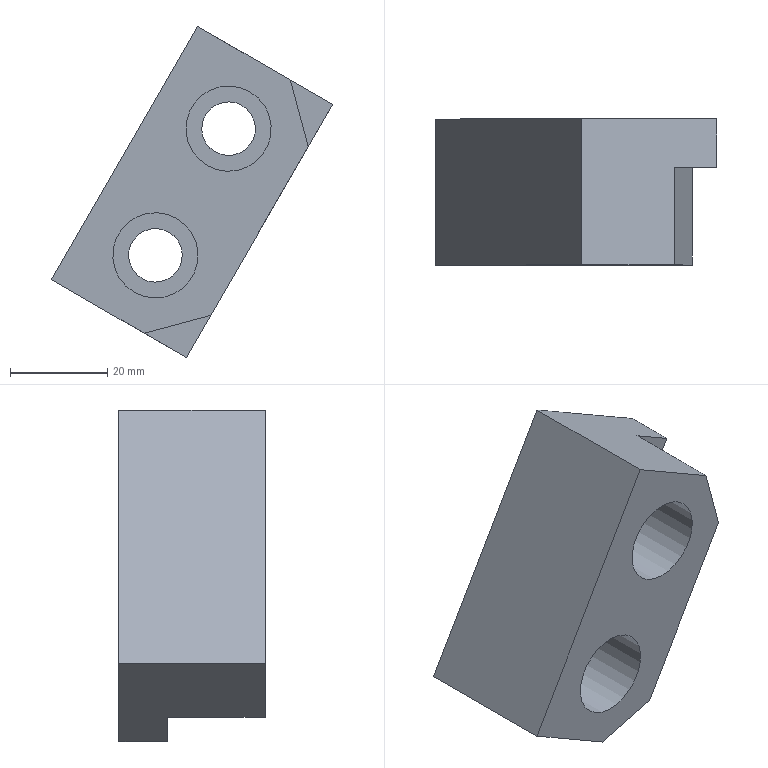Part | NX | features solid 2 | 1 solid | 16 faces | box 57.713 x 30 x 67.962 mm | volume 44078 mm3 | plane 12 | cylinder 4 | commonest cylinder face diameters 11 x2 17.5 x2
STEP:
#1=CARTESIAN_POINT('',(360.44,-388.,-19.66));
#2=VERTEX_POINT('',#1);
#3=CARTESIAN_POINT('',(360.44,-368.,-19.66));
#4=VERTEX_POINT('',#3);
#5=CARTESIAN_POINT('',(360.44,-388.,-19.66));
#6=DIRECTION('',(0.,-1.,0.));
#7=VECTOR('',#6,1000.);
#8=LINE('',#5,#7);
#9=EDGE_CURVE('',#2,#4,#8,.F.);
#10=ORIENTED_EDGE('',*,*,#9,.F.);
#11=CARTESIAN_POINT('',(340.44,-388.,-54.301));
#12=VERTEX_POINT('',#11);
#13=CARTESIAN_POINT('',(365.44,-388.,-11.));
#14=DIRECTION('',(-0.5,0.,-0.866));
#15=VECTOR('',#14,1000.);
#16=LINE('',#13,#15);
#17=EDGE_CURVE('',#2,#12,#16,.T.);
#18=ORIENTED_EDGE('',*,*,#17,.T.);
#19=CARTESIAN_POINT('',(340.44,-368.,-54.301));
#20=VERTEX_POINT('',#19);
#21=CARTESIAN_POINT('',(340.44,-388.,-54.301));
#22=DIRECTION('',(0.,1.,0.));
#23=VECTOR('',#22,1000.);
#24=LINE('',#21,#23);
#25=EDGE_CURVE('',#12,#20,#24,.T.);
#26=ORIENTED_EDGE('',*,*,#25,.T.);
#27=CARTESIAN_POINT('',(335.44,-368.,-62.962));
#28=VERTEX_POINT('',#27);
#29=CARTESIAN_POINT('',(365.44,-368.,-11.));
#30=DIRECTION('',(-0.5,0.,-0.866));
#31=VECTOR('',#30,1000.);
#32=LINE('',#29,#31);
#33=EDGE_CURVE('',#28,#20,#32,.F.);
#34=ORIENTED_EDGE('',*,*,#33,.F.);
#35=CARTESIAN_POINT('',(335.44,-358.,-62.962));
#36=VERTEX_POINT('',#35);
#37=CARTESIAN_POINT('',(335.44,-388.,-62.962));
#38=DIRECTION('',(0.,-1.,0.));
#39=VECTOR('',#38,1000.);
#40=LINE('',#37,#39);
#41=EDGE_CURVE('',#28,#36,#40,.F.);
#42=ORIENTED_EDGE('',*,*,#41,.T.);
#43=CARTESIAN_POINT('',(365.44,-358.,-11.));
#44=VERTEX_POINT('',#43);
#45=CARTESIAN_POINT('',(365.44,-358.,-11.));
#46=DIRECTION('',(-0.5,0.,-0.866));
#47=VECTOR('',#46,1000.);
#48=LINE('',#45,#47);
#49=EDGE_CURVE('',#44,#36,#48,.T.);
#50=ORIENTED_EDGE('',*,*,#49,.F.);
#51=CARTESIAN_POINT('',(365.44,-368.,-11.));
#52=VERTEX_POINT('',#51);
#53=CARTESIAN_POINT('',(365.44,-388.,-11.));
#54=DIRECTION('',(0.,-1.,0.));
#55=VECTOR('',#54,1000.);
#56=LINE('',#53,#55);
#57=EDGE_CURVE('',#52,#44,#56,.F.);
#58=ORIENTED_EDGE('',*,*,#57,.F.);
#59=CARTESIAN_POINT('',(365.44,-368.,-11.));
#60=DIRECTION('',(0.5,0.,0.866));
#61=VECTOR('',#60,1000.);
#62=LINE('',#59,#61);
#63=EDGE_CURVE('',#52,#4,#62,.F.);
#64=ORIENTED_EDGE('',*,*,#63,.T.);
#65=EDGE_LOOP('',(#10,#18,#26,#34,#42,#50,#58,#64));
#66=FACE_BOUND('',#65,.T.);
#67=CARTESIAN_POINT('',(365.44,-388.,-11.));
#68=DIRECTION('',(0.866,0.,-0.5));
#69=DIRECTION('',(-0.5,0.,-0.866));
#70=AXIS2_PLACEMENT_3D('',#67,#68,#69);
#71=PLANE('',#70);
#72=ADVANCED_FACE('',(#66),#71,.T.);
#73=CARTESIAN_POINT('',(356.779,-388.,-6.));
#74=VERTEX_POINT('',#73);
#75=CARTESIAN_POINT('',(356.779,-368.,-6.));
#76=VERTEX_POINT('',#75);
#77=CARTESIAN_POINT('',(356.779,-388.,-6.));
#78=DIRECTION('',(0.,-1.,0.));
#79=VECTOR('',#78,1000.);
#80=LINE('',#77,#79);
#81=EDGE_CURVE('',#74,#76,#80,.F.);
#82=ORIENTED_EDGE('',*,*,#81,.T.);
#83=CARTESIAN_POINT('',(365.44,-368.,-11.));
#84=DIRECTION('',(0.866,0.,-0.5));
#85=VECTOR('',#84,1000.);
#86=LINE('',#83,#85);
#87=EDGE_CURVE('',#76,#52,#86,.T.);
#88=ORIENTED_EDGE('',*,*,#87,.T.);
#89=ORIENTED_EDGE('',*,*,#57,.T.);
#90=CARTESIAN_POINT('',(337.727,-358.,5.));
#91=VERTEX_POINT('',#90);
#92=CARTESIAN_POINT('',(365.44,-358.,-11.));
#93=DIRECTION('',(-0.866,0.,0.5));
#94=VECTOR('',#93,1000.);
#95=LINE('',#92,#94);
#96=EDGE_CURVE('',#44,#91,#95,.T.);
#97=ORIENTED_EDGE('',*,*,#96,.T.);
#98=CARTESIAN_POINT('',(337.727,-388.,5.));
#99=VERTEX_POINT('',#98);
#100=CARTESIAN_POINT('',(337.727,-388.,5.));
#101=DIRECTION('',(0.,1.,0.));
#102=VECTOR('',#101,1000.);
#103=LINE('',#100,#102);
#104=EDGE_CURVE('',#99,#91,#103,.T.);
#105=ORIENTED_EDGE('',*,*,#104,.F.);
#106=CARTESIAN_POINT('',(365.44,-388.,-11.));
#107=DIRECTION('',(-0.866,0.,0.5));
#108=VECTOR('',#107,1000.);
#109=LINE('',#106,#108);
#110=EDGE_CURVE('',#74,#99,#109,.T.);
#111=ORIENTED_EDGE('',*,*,#110,.F.);
#112=EDGE_LOOP('',(#82,#88,#89,#97,#105,#111));
#113=FACE_BOUND('',#112,.T.);
#114=CARTESIAN_POINT('',(365.44,-388.,-11.));
#115=DIRECTION('',(-0.5,0.,-0.866));
#116=DIRECTION('',(-0.866,0.,0.5));
#117=AXIS2_PLACEMENT_3D('',#114,#115,#116);
#118=PLANE('',#117);
#119=ADVANCED_FACE('',(#113),#118,.F.);
#120=CARTESIAN_POINT('',(348.458,-388.,-8.413));
#121=VERTEX_POINT('',#120);
#122=CARTESIAN_POINT('',(344.083,-388.,-15.99));
#123=DIRECTION('',(0.,-1.,0.));
#124=DIRECTION('',(0.5,0.,0.866));
#125=AXIS2_PLACEMENT_3D('',#122,#123,#124);
#126=CIRCLE('',#125,8.75);
#127=EDGE_CURVE('',#121,#121,#126,.T.);
#128=ORIENTED_EDGE('',*,*,#127,.F.);
#129=EDGE_LOOP('',(#128));
#130=FACE_BOUND('',#129,.T.);
#131=CARTESIAN_POINT('',(333.458,-388.,-34.393));
#132=VERTEX_POINT('',#131);
#133=CARTESIAN_POINT('',(329.083,-388.,-41.971));
#134=DIRECTION('',(0.,-1.,0.));
#135=DIRECTION('',(0.5,0.,0.866));
#136=AXIS2_PLACEMENT_3D('',#133,#134,#135);
#137=CIRCLE('',#136,8.75);
#138=EDGE_CURVE('',#132,#132,#137,.T.);
#139=ORIENTED_EDGE('',*,*,#138,.F.);
#140=EDGE_LOOP('',(#139));
#141=FACE_BOUND('',#140,.T.);
#142=ORIENTED_EDGE('',*,*,#110,.T.);
#143=CARTESIAN_POINT('',(307.727,-388.,-46.962));
#144=VERTEX_POINT('',#143);
#145=CARTESIAN_POINT('',(337.727,-388.,5.));
#146=DIRECTION('',(-0.5,0.,-0.866));
#147=VECTOR('',#146,1000.);
#148=LINE('',#145,#147);
#149=EDGE_CURVE('',#99,#144,#148,.T.);
#150=ORIENTED_EDGE('',*,*,#149,.T.);
#151=CARTESIAN_POINT('',(326.779,-388.,-57.962));
#152=VERTEX_POINT('',#151);
#153=CARTESIAN_POINT('',(335.44,-388.,-62.962));
#154=DIRECTION('',(-0.866,0.,0.5));
#155=VECTOR('',#154,1000.);
#156=LINE('',#153,#155);
#157=EDGE_CURVE('',#152,#144,#156,.T.);
#158=ORIENTED_EDGE('',*,*,#157,.F.);
#159=CARTESIAN_POINT('',(340.44,-388.,-54.301));
#160=DIRECTION('',(-0.9659,0.,-0.2588));
#161=VECTOR('',#160,1000.);
#162=LINE('',#159,#161);
#163=EDGE_CURVE('',#12,#152,#162,.T.);
#164=ORIENTED_EDGE('',*,*,#163,.F.);
#165=ORIENTED_EDGE('',*,*,#17,.F.);
#166=CARTESIAN_POINT('',(360.44,-388.,-19.66));
#167=DIRECTION('',(-0.2588,0.,0.9659));
#168=VECTOR('',#167,1000.);
#169=LINE('',#166,#168);
#170=EDGE_CURVE('',#2,#74,#169,.T.);
#171=ORIENTED_EDGE('',*,*,#170,.T.);
#172=EDGE_LOOP('',(#142,#150,#158,#164,#165,#171));
#173=FACE_BOUND('',#172,.T.);
#174=CARTESIAN_POINT('',(365.44,-388.,-11.));
#175=DIRECTION('',(0.,-1.,0.));
#176=DIRECTION('',(-0.5,0.,-0.866));
#177=AXIS2_PLACEMENT_3D('',#174,#175,#176);
#178=PLANE('',#177);
#179=ADVANCED_FACE('',(#130,#141,#173),#178,.T.);
#180=ORIENTED_EDGE('',*,*,#157,.T.);
#181=CARTESIAN_POINT('',(307.727,-358.,-46.962));
#182=VERTEX_POINT('',#181);
#183=CARTESIAN_POINT('',(307.727,-388.,-46.962));
#184=DIRECTION('',(0.,-1.,0.));
#185=VECTOR('',#184,1000.);
#186=LINE('',#183,#185);
#187=EDGE_CURVE('',#144,#182,#186,.F.);
#188=ORIENTED_EDGE('',*,*,#187,.T.);
#189=CARTESIAN_POINT('',(335.44,-358.,-62.962));
#190=DIRECTION('',(-0.866,0.,0.5));
#191=VECTOR('',#190,1000.);
#192=LINE('',#189,#191);
#193=EDGE_CURVE('',#36,#182,#192,.T.);
#194=ORIENTED_EDGE('',*,*,#193,.F.);
#195=ORIENTED_EDGE('',*,*,#41,.F.);
#196=CARTESIAN_POINT('',(326.779,-368.,-57.962));
#197=VERTEX_POINT('',#196);
#198=CARTESIAN_POINT('',(335.44,-368.,-62.962));
#199=DIRECTION('',(-0.866,0.,0.5));
#200=VECTOR('',#199,1000.);
#201=LINE('',#198,#200);
#202=EDGE_CURVE('',#197,#28,#201,.F.);
#203=ORIENTED_EDGE('',*,*,#202,.F.);
#204=CARTESIAN_POINT('',(326.779,-388.,-57.962));
#205=DIRECTION('',(0.,-1.,0.));
#206=VECTOR('',#205,1000.);
#207=LINE('',#204,#206);
#208=EDGE_CURVE('',#152,#197,#207,.F.);
#209=ORIENTED_EDGE('',*,*,#208,.F.);
#210=EDGE_LOOP('',(#180,#188,#194,#195,#203,#209));
#211=FACE_BOUND('',#210,.T.);
#212=CARTESIAN_POINT('',(335.44,-388.,-62.962));
#213=DIRECTION('',(-0.5,0.,-0.866));
#214=DIRECTION('',(-0.866,0.,0.5));
#215=AXIS2_PLACEMENT_3D('',#212,#213,#214);
#216=PLANE('',#215);
#217=ADVANCED_FACE('',(#211),#216,.T.);
#218=ORIENTED_EDGE('',*,*,#187,.F.);
#219=ORIENTED_EDGE('',*,*,#149,.F.);
#220=ORIENTED_EDGE('',*,*,#104,.T.);
#221=CARTESIAN_POINT('',(337.727,-358.,5.));
#222=DIRECTION('',(-0.5,0.,-0.866));
#223=VECTOR('',#222,1000.);
#224=LINE('',#221,#223);
#225=EDGE_CURVE('',#91,#182,#224,.T.);
#226=ORIENTED_EDGE('',*,*,#225,.T.);
#227=EDGE_LOOP('',(#218,#219,#220,#226));
#228=FACE_BOUND('',#227,.T.);
#229=CARTESIAN_POINT('',(337.727,-388.,5.));
#230=DIRECTION('',(0.866,0.,-0.5));
#231=DIRECTION('',(-0.5,0.,-0.866));
#232=AXIS2_PLACEMENT_3D('',#229,#230,#231);
#233=PLANE('',#232);
#234=ADVANCED_FACE('',(#228),#233,.F.);
#235=CARTESIAN_POINT('',(326.333,-358.,-46.734));
#236=VERTEX_POINT('',#235);
#237=CARTESIAN_POINT('',(329.083,-358.,-41.971));
#238=DIRECTION('',(0.,1.,0.));
#239=DIRECTION('',(-0.5,0.,-0.866));
#240=AXIS2_PLACEMENT_3D('',#237,#238,#239);
#241=CIRCLE('',#240,5.5);
#242=EDGE_CURVE('',#236,#236,#241,.T.);
#243=ORIENTED_EDGE('',*,*,#242,.F.);
#244=EDGE_LOOP('',(#243));
#245=FACE_BOUND('',#244,.T.);
#246=CARTESIAN_POINT('',(341.333,-358.,-20.754));
#247=VERTEX_POINT('',#246);
#248=CARTESIAN_POINT('',(344.083,-358.,-15.99));
#249=DIRECTION('',(0.,1.,0.));
#250=DIRECTION('',(-0.5,0.,-0.866));
#251=AXIS2_PLACEMENT_3D('',#248,#249,#250);
#252=CIRCLE('',#251,5.5);
#253=EDGE_CURVE('',#247,#247,#252,.T.);
#254=ORIENTED_EDGE('',*,*,#253,.F.);
#255=EDGE_LOOP('',(#254));
#256=FACE_BOUND('',#255,.T.);
#257=ORIENTED_EDGE('',*,*,#225,.F.);
#258=ORIENTED_EDGE('',*,*,#96,.F.);
#259=ORIENTED_EDGE('',*,*,#49,.T.);
#260=ORIENTED_EDGE('',*,*,#193,.T.);
#261=EDGE_LOOP('',(#257,#258,#259,#260));
#262=FACE_BOUND('',#261,.T.);
#263=CARTESIAN_POINT('',(365.44,-358.,-11.));
#264=DIRECTION('',(0.,-1.,0.));
#265=DIRECTION('',(-0.5,0.,-0.866));
#266=AXIS2_PLACEMENT_3D('',#263,#264,#265);
#267=PLANE('',#266);
#268=ADVANCED_FACE('',(#245,#256,#262),#267,.F.);
#269=CARTESIAN_POINT('',(346.833,-368.,-11.227));
#270=VERTEX_POINT('',#269);
#271=CARTESIAN_POINT('',(344.083,-368.,-15.99));
#272=DIRECTION('',(0.,-1.,0.));
#273=DIRECTION('',(0.5,0.,0.866));
#274=AXIS2_PLACEMENT_3D('',#271,#272,#273);
#275=CIRCLE('',#274,5.5);
#276=EDGE_CURVE('',#270,#270,#275,.T.);
#277=ORIENTED_EDGE('',*,*,#276,.T.);
#278=EDGE_LOOP('',(#277));
#279=FACE_BOUND('',#278,.T.);
#280=ORIENTED_EDGE('',*,*,#253,.T.);
#281=EDGE_LOOP('',(#280));
#282=FACE_BOUND('',#281,.T.);
#283=CARTESIAN_POINT('',(344.083,-288.,-15.99));
#284=DIRECTION('',(0.,1.,0.));
#285=DIRECTION('',(0.5,0.,0.866));
#286=AXIS2_PLACEMENT_3D('',#283,#284,#285);
#287=CYLINDRICAL_SURFACE('',#286,5.5);
#288=ADVANCED_FACE('',(#279,#282),#287,.F.);
#289=ORIENTED_EDGE('',*,*,#276,.F.);
#290=EDGE_LOOP('',(#289));
#291=FACE_BOUND('',#290,.T.);
#292=CARTESIAN_POINT('',(348.458,-368.,-8.413));
#293=VERTEX_POINT('',#292);
#294=CARTESIAN_POINT('',(344.083,-368.,-15.99));
#295=DIRECTION('',(0.,-1.,0.));
#296=DIRECTION('',(0.5,0.,0.866));
#297=AXIS2_PLACEMENT_3D('',#294,#295,#296);
#298=CIRCLE('',#297,8.75);
#299=EDGE_CURVE('',#293,#293,#298,.T.);
#300=ORIENTED_EDGE('',*,*,#299,.T.);
#301=EDGE_LOOP('',(#300));
#302=FACE_BOUND('',#301,.T.);
#303=CARTESIAN_POINT('',(344.083,-368.,-15.99));
#304=DIRECTION('',(0.,1.,0.));
#305=DIRECTION('',(0.5,0.,0.866));
#306=AXIS2_PLACEMENT_3D('',#303,#304,#305);
#307=PLANE('',#306);
#308=ADVANCED_FACE('',(#291,#302),#307,.F.);
#309=ORIENTED_EDGE('',*,*,#299,.F.);
#310=EDGE_LOOP('',(#309));
#311=FACE_BOUND('',#310,.T.);
#312=ORIENTED_EDGE('',*,*,#127,.T.);
#313=EDGE_LOOP('',(#312));
#314=FACE_BOUND('',#313,.T.);
#315=CARTESIAN_POINT('',(344.083,-388.,-15.99));
#316=DIRECTION('',(0.,1.,0.));
#317=DIRECTION('',(0.5,0.,0.866));
#318=AXIS2_PLACEMENT_3D('',#315,#316,#317);
#319=CYLINDRICAL_SURFACE('',#318,8.75);
#320=ADVANCED_FACE('',(#311,#314),#319,.F.);
#321=CARTESIAN_POINT('',(331.833,-368.,-37.208));
#322=VERTEX_POINT('',#321);
#323=CARTESIAN_POINT('',(329.083,-368.,-41.971));
#324=DIRECTION('',(0.,-1.,0.));
#325=DIRECTION('',(0.5,0.,0.866));
#326=AXIS2_PLACEMENT_3D('',#323,#324,#325);
#327=CIRCLE('',#326,5.5);
#328=EDGE_CURVE('',#322,#322,#327,.T.);
#329=ORIENTED_EDGE('',*,*,#328,.T.);
#330=EDGE_LOOP('',(#329));
#331=FACE_BOUND('',#330,.T.);
#332=ORIENTED_EDGE('',*,*,#242,.T.);
#333=EDGE_LOOP('',(#332));
#334=FACE_BOUND('',#333,.T.);
#335=CARTESIAN_POINT('',(329.083,-288.,-41.971));
#336=DIRECTION('',(0.,1.,0.));
#337=DIRECTION('',(0.5,0.,0.866));
#338=AXIS2_PLACEMENT_3D('',#335,#336,#337);
#339=CYLINDRICAL_SURFACE('',#338,5.5);
#340=ADVANCED_FACE('',(#331,#334),#339,.F.);
#341=ORIENTED_EDGE('',*,*,#328,.F.);
#342=EDGE_LOOP('',(#341));
#343=FACE_BOUND('',#342,.T.);
#344=CARTESIAN_POINT('',(333.458,-368.,-34.393));
#345=VERTEX_POINT('',#344);
#346=CARTESIAN_POINT('',(329.083,-368.,-41.971));
#347=DIRECTION('',(0.,-1.,0.));
#348=DIRECTION('',(0.5,0.,0.866));
#349=AXIS2_PLACEMENT_3D('',#346,#347,#348);
#350=CIRCLE('',#349,8.75);
#351=EDGE_CURVE('',#345,#345,#350,.T.);
#352=ORIENTED_EDGE('',*,*,#351,.T.);
#353=EDGE_LOOP('',(#352));
#354=FACE_BOUND('',#353,.T.);
#355=CARTESIAN_POINT('',(329.083,-368.,-41.971));
#356=DIRECTION('',(0.,1.,0.));
#357=DIRECTION('',(0.5,0.,0.866));
#358=AXIS2_PLACEMENT_3D('',#355,#356,#357);
#359=PLANE('',#358);
#360=ADVANCED_FACE('',(#343,#354),#359,.F.);
#361=ORIENTED_EDGE('',*,*,#351,.F.);
#362=EDGE_LOOP('',(#361));
#363=FACE_BOUND('',#362,.T.);
#364=ORIENTED_EDGE('',*,*,#138,.T.);
#365=EDGE_LOOP('',(#364));
#366=FACE_BOUND('',#365,.T.);
#367=CARTESIAN_POINT('',(329.083,-388.,-41.971));
#368=DIRECTION('',(0.,1.,0.));
#369=DIRECTION('',(0.5,0.,0.866));
#370=AXIS2_PLACEMENT_3D('',#367,#368,#369);
#371=CYLINDRICAL_SURFACE('',#370,8.75);
#372=ADVANCED_FACE('',(#363,#366),#371,.F.);
#373=ORIENTED_EDGE('',*,*,#202,.T.);
#374=ORIENTED_EDGE('',*,*,#33,.T.);
#375=CARTESIAN_POINT('',(340.44,-368.,-54.301));
#376=DIRECTION('',(-0.9659,0.,-0.2588));
#377=VECTOR('',#376,1000.);
#378=LINE('',#375,#377);
#379=EDGE_CURVE('',#20,#197,#378,.T.);
#380=ORIENTED_EDGE('',*,*,#379,.T.);
#381=EDGE_LOOP('',(#373,#374,#380));
#382=FACE_BOUND('',#381,.T.);
#383=CARTESIAN_POINT('',(340.44,-368.,-54.301));
#384=DIRECTION('',(0.,1.,0.));
#385=DIRECTION('',(0.5,0.,0.866));
#386=AXIS2_PLACEMENT_3D('',#383,#384,#385);
#387=PLANE('',#386);
#388=ADVANCED_FACE('',(#382),#387,.F.);
#389=ORIENTED_EDGE('',*,*,#163,.T.);
#390=ORIENTED_EDGE('',*,*,#208,.T.);
#391=ORIENTED_EDGE('',*,*,#379,.F.);
#392=ORIENTED_EDGE('',*,*,#25,.F.);
#393=EDGE_LOOP('',(#389,#390,#391,#392));
#394=FACE_BOUND('',#393,.T.);
#395=CARTESIAN_POINT('',(340.44,-388.,-54.301));
#396=DIRECTION('',(-0.2588,0.,0.9659));
#397=DIRECTION('',(-0.9659,0.,-0.2588));
#398=AXIS2_PLACEMENT_3D('',#395,#396,#397);
#399=PLANE('',#398);
#400=ADVANCED_FACE('',(#394),#399,.F.);
#401=ORIENTED_EDGE('',*,*,#63,.F.);
#402=ORIENTED_EDGE('',*,*,#87,.F.);
#403=CARTESIAN_POINT('',(360.44,-368.,-19.66));
#404=DIRECTION('',(-0.2588,0.,0.9659));
#405=VECTOR('',#404,1000.);
#406=LINE('',#403,#405);
#407=EDGE_CURVE('',#4,#76,#406,.T.);
#408=ORIENTED_EDGE('',*,*,#407,.F.);
#409=EDGE_LOOP('',(#401,#402,#408));
#410=FACE_BOUND('',#409,.T.);
#411=CARTESIAN_POINT('',(360.44,-368.,-19.66));
#412=DIRECTION('',(0.,-1.,0.));
#413=DIRECTION('',(-0.5,0.,-0.866));
#414=AXIS2_PLACEMENT_3D('',#411,#412,#413);
#415=PLANE('',#414);
#416=ADVANCED_FACE('',(#410),#415,.T.);
#417=ORIENTED_EDGE('',*,*,#81,.F.);
#418=ORIENTED_EDGE('',*,*,#170,.F.);
#419=ORIENTED_EDGE('',*,*,#9,.T.);
#420=ORIENTED_EDGE('',*,*,#407,.T.);
#421=EDGE_LOOP('',(#417,#418,#419,#420));
#422=FACE_BOUND('',#421,.T.);
#423=CARTESIAN_POINT('',(360.44,-388.,-19.66));
#424=DIRECTION('',(-0.9659,0.,-0.2588));
#425=DIRECTION('',(-0.2588,0.,0.9659));
#426=AXIS2_PLACEMENT_3D('',#423,#424,#425);
#427=PLANE('',#426);
#428=ADVANCED_FACE('',(#422),#427,.F.);
#429=CLOSED_SHELL('',(#72,#119,#179,#217,#234,#268,#288,#308,#320,#340,#360,#372,#388,#400,#416,#428));
#430=MANIFOLD_SOLID_BREP('',#429);
#431=(LENGTH_UNIT()NAMED_UNIT(*)SI_UNIT(.MILLI.,.METRE.));
#432=UNCERTAINTY_MEASURE_WITH_UNIT(LENGTH_MEASURE(0.00001),#431,'','');
#433=(NAMED_UNIT(*)PLANE_ANGLE_UNIT()SI_UNIT($,.RADIAN.));
#434=(NAMED_UNIT(*)SI_UNIT($,.STERADIAN.)SOLID_ANGLE_UNIT());
#435=(GEOMETRIC_REPRESENTATION_CONTEXT(3)GLOBAL_UNCERTAINTY_ASSIGNED_CONTEXT((#432))GLOBAL_UNIT_ASSIGNED_CONTEXT((#431,#433,#434))REPRESENTATION_CONTEXT('',''));
#436=ADVANCED_BREP_SHAPE_REPRESENTATION('',(#430),#435);